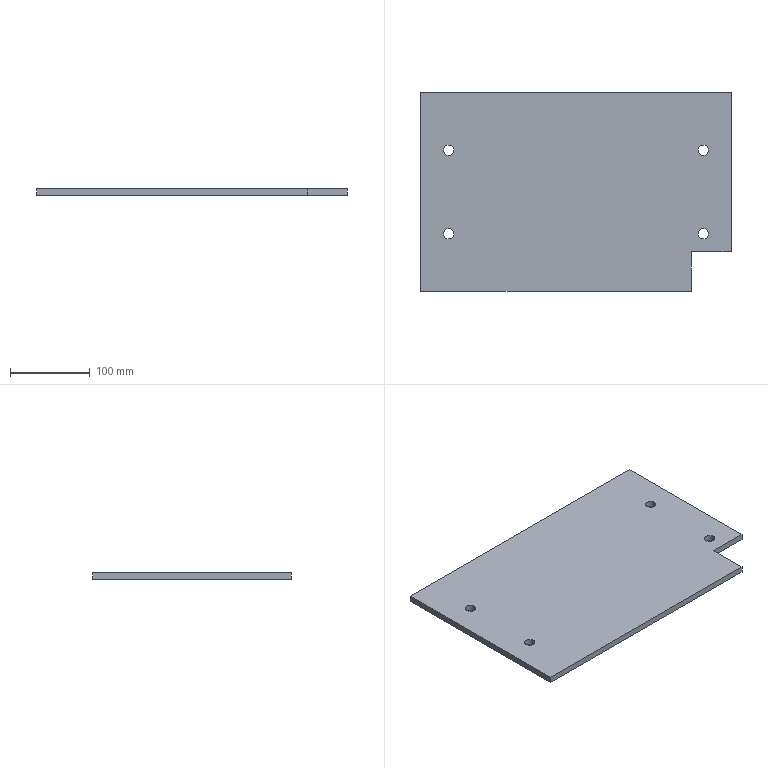Part | SolidWorks | features ICE 2, Extrusion 1 | 1 solid | 16 faces | box 390 x 250 x 8 mm | volume 755753 mm3 | cylinder 8 | plane 8 | commonest cylinder face diameters 13 x8
STEP:
#1=CARTESIAN_POINT('',(348.5,177.5,0.));
#2=VERTEX_POINT('',#1);
#3=CARTESIAN_POINT('',(361.5,177.5,0.));
#4=VERTEX_POINT('',#3);
#5=CARTESIAN_POINT('',(355.,177.5,0.));
#6=DIRECTION('',(0.,0.,1.));
#7=DIRECTION('',(1.,0.,0.));
#8=AXIS2_PLACEMENT_3D('',#5,#6,#7);
#9=CIRCLE('',#8,6.5);
#10=EDGE_CURVE('',#2,#4,#9,.T.);
#11=ORIENTED_EDGE('',*,*,#10,.F.);
#12=CARTESIAN_POINT('',(348.5,177.5,8.));
#13=VERTEX_POINT('',#12);
#14=CARTESIAN_POINT('',(348.5,177.5,0.));
#15=DIRECTION('',(0.,0.,1.));
#16=VECTOR('',#15,1000.);
#17=LINE('',#14,#16);
#18=EDGE_CURVE('',#2,#13,#17,.T.);
#19=ORIENTED_EDGE('',*,*,#18,.T.);
#20=CARTESIAN_POINT('',(361.5,177.5,8.));
#21=VERTEX_POINT('',#20);
#22=CARTESIAN_POINT('',(355.,177.5,8.));
#23=DIRECTION('',(0.,0.,1.));
#24=DIRECTION('',(1.,0.,0.));
#25=AXIS2_PLACEMENT_3D('',#22,#23,#24);
#26=CIRCLE('',#25,6.5);
#27=EDGE_CURVE('',#13,#21,#26,.T.);
#28=ORIENTED_EDGE('',*,*,#27,.T.);
#29=CARTESIAN_POINT('',(361.5,177.5,0.));
#30=DIRECTION('',(0.,0.,1.));
#31=VECTOR('',#30,1000.);
#32=LINE('',#29,#31);
#33=EDGE_CURVE('',#4,#21,#32,.T.);
#34=ORIENTED_EDGE('',*,*,#33,.F.);
#35=EDGE_LOOP('',(#11,#19,#28,#34));
#36=FACE_OUTER_BOUND('',#35,.T.);
#37=CARTESIAN_POINT('',(355.,177.5,0.));
#38=DIRECTION('',(0.,0.,1.));
#39=DIRECTION('',(1.,0.,0.));
#40=AXIS2_PLACEMENT_3D('',#37,#38,#39);
#41=CYLINDRICAL_SURFACE('',#40,6.5);
#42=ADVANCED_FACE('',(#36),#41,.F.);
#43=CARTESIAN_POINT('',(348.5,72.5,0.));
#44=VERTEX_POINT('',#43);
#45=CARTESIAN_POINT('',(361.5,72.5,0.));
#46=VERTEX_POINT('',#45);
#47=CARTESIAN_POINT('',(355.,72.5,0.));
#48=DIRECTION('',(0.,0.,1.));
#49=DIRECTION('',(1.,0.,0.));
#50=AXIS2_PLACEMENT_3D('',#47,#48,#49);
#51=CIRCLE('',#50,6.5);
#52=EDGE_CURVE('',#44,#46,#51,.T.);
#53=ORIENTED_EDGE('',*,*,#52,.F.);
#54=CARTESIAN_POINT('',(348.5,72.5,8.));
#55=VERTEX_POINT('',#54);
#56=CARTESIAN_POINT('',(348.5,72.5,0.));
#57=DIRECTION('',(0.,0.,1.));
#58=VECTOR('',#57,1000.);
#59=LINE('',#56,#58);
#60=EDGE_CURVE('',#44,#55,#59,.T.);
#61=ORIENTED_EDGE('',*,*,#60,.T.);
#62=CARTESIAN_POINT('',(361.5,72.5,8.));
#63=VERTEX_POINT('',#62);
#64=CARTESIAN_POINT('',(355.,72.5,8.));
#65=DIRECTION('',(0.,0.,1.));
#66=DIRECTION('',(1.,0.,0.));
#67=AXIS2_PLACEMENT_3D('',#64,#65,#66);
#68=CIRCLE('',#67,6.5);
#69=EDGE_CURVE('',#55,#63,#68,.T.);
#70=ORIENTED_EDGE('',*,*,#69,.T.);
#71=CARTESIAN_POINT('',(361.5,72.5,0.));
#72=DIRECTION('',(0.,0.,1.));
#73=VECTOR('',#72,1000.);
#74=LINE('',#71,#73);
#75=EDGE_CURVE('',#46,#63,#74,.T.);
#76=ORIENTED_EDGE('',*,*,#75,.F.);
#77=EDGE_LOOP('',(#53,#61,#70,#76));
#78=FACE_OUTER_BOUND('',#77,.T.);
#79=CARTESIAN_POINT('',(355.,72.5,0.));
#80=DIRECTION('',(0.,0.,1.));
#81=DIRECTION('',(1.,0.,0.));
#82=AXIS2_PLACEMENT_3D('',#79,#80,#81);
#83=CYLINDRICAL_SURFACE('',#82,6.5);
#84=ADVANCED_FACE('',(#78),#83,.F.);
#85=CARTESIAN_POINT('',(28.5,72.5,0.));
#86=VERTEX_POINT('',#85);
#87=CARTESIAN_POINT('',(41.5,72.5,0.));
#88=VERTEX_POINT('',#87);
#89=CARTESIAN_POINT('',(35.,72.5,0.));
#90=DIRECTION('',(0.,0.,1.));
#91=DIRECTION('',(1.,0.,0.));
#92=AXIS2_PLACEMENT_3D('',#89,#90,#91);
#93=CIRCLE('',#92,6.5);
#94=EDGE_CURVE('',#86,#88,#93,.T.);
#95=ORIENTED_EDGE('',*,*,#94,.F.);
#96=CARTESIAN_POINT('',(28.5,72.5,8.));
#97=VERTEX_POINT('',#96);
#98=CARTESIAN_POINT('',(28.5,72.5,0.));
#99=DIRECTION('',(0.,0.,1.));
#100=VECTOR('',#99,1000.);
#101=LINE('',#98,#100);
#102=EDGE_CURVE('',#86,#97,#101,.T.);
#103=ORIENTED_EDGE('',*,*,#102,.T.);
#104=CARTESIAN_POINT('',(41.5,72.5,8.));
#105=VERTEX_POINT('',#104);
#106=CARTESIAN_POINT('',(35.,72.5,8.));
#107=DIRECTION('',(0.,0.,1.));
#108=DIRECTION('',(1.,0.,0.));
#109=AXIS2_PLACEMENT_3D('',#106,#107,#108);
#110=CIRCLE('',#109,6.5);
#111=EDGE_CURVE('',#97,#105,#110,.T.);
#112=ORIENTED_EDGE('',*,*,#111,.T.);
#113=CARTESIAN_POINT('',(41.5,72.5,0.));
#114=DIRECTION('',(0.,0.,1.));
#115=VECTOR('',#114,1000.);
#116=LINE('',#113,#115);
#117=EDGE_CURVE('',#88,#105,#116,.T.);
#118=ORIENTED_EDGE('',*,*,#117,.F.);
#119=EDGE_LOOP('',(#95,#103,#112,#118));
#120=FACE_OUTER_BOUND('',#119,.T.);
#121=CARTESIAN_POINT('',(35.,72.5,0.));
#122=DIRECTION('',(0.,0.,1.));
#123=DIRECTION('',(1.,0.,0.));
#124=AXIS2_PLACEMENT_3D('',#121,#122,#123);
#125=CYLINDRICAL_SURFACE('',#124,6.5);
#126=ADVANCED_FACE('',(#120),#125,.F.);
#127=CARTESIAN_POINT('',(28.5,177.5,0.));
#128=VERTEX_POINT('',#127);
#129=CARTESIAN_POINT('',(41.5,177.5,0.));
#130=VERTEX_POINT('',#129);
#131=CARTESIAN_POINT('',(35.,177.5,0.));
#132=DIRECTION('',(0.,0.,1.));
#133=DIRECTION('',(1.,0.,0.));
#134=AXIS2_PLACEMENT_3D('',#131,#132,#133);
#135=CIRCLE('',#134,6.5);
#136=EDGE_CURVE('',#128,#130,#135,.T.);
#137=ORIENTED_EDGE('',*,*,#136,.F.);
#138=CARTESIAN_POINT('',(28.5,177.5,8.));
#139=VERTEX_POINT('',#138);
#140=CARTESIAN_POINT('',(28.5,177.5,0.));
#141=DIRECTION('',(0.,0.,1.));
#142=VECTOR('',#141,1000.);
#143=LINE('',#140,#142);
#144=EDGE_CURVE('',#128,#139,#143,.T.);
#145=ORIENTED_EDGE('',*,*,#144,.T.);
#146=CARTESIAN_POINT('',(41.5,177.5,8.));
#147=VERTEX_POINT('',#146);
#148=CARTESIAN_POINT('',(35.,177.5,8.));
#149=DIRECTION('',(0.,0.,1.));
#150=DIRECTION('',(1.,0.,0.));
#151=AXIS2_PLACEMENT_3D('',#148,#149,#150);
#152=CIRCLE('',#151,6.5);
#153=EDGE_CURVE('',#139,#147,#152,.T.);
#154=ORIENTED_EDGE('',*,*,#153,.T.);
#155=CARTESIAN_POINT('',(41.5,177.5,0.));
#156=DIRECTION('',(0.,0.,1.));
#157=VECTOR('',#156,1000.);
#158=LINE('',#155,#157);
#159=EDGE_CURVE('',#130,#147,#158,.T.);
#160=ORIENTED_EDGE('',*,*,#159,.F.);
#161=EDGE_LOOP('',(#137,#145,#154,#160));
#162=FACE_OUTER_BOUND('',#161,.T.);
#163=CARTESIAN_POINT('',(35.,177.5,0.));
#164=DIRECTION('',(0.,0.,1.));
#165=DIRECTION('',(1.,0.,0.));
#166=AXIS2_PLACEMENT_3D('',#163,#164,#165);
#167=CYLINDRICAL_SURFACE('',#166,6.5);
#168=ADVANCED_FACE('',(#162),#167,.F.);
#169=CARTESIAN_POINT('',(0.,0.,0.));
#170=VERTEX_POINT('',#169);
#171=CARTESIAN_POINT('',(340.,0.,0.));
#172=VERTEX_POINT('',#171);
#173=CARTESIAN_POINT('',(390.,0.,0.));
#174=DIRECTION('',(1.,0.,0.));
#175=VECTOR('',#174,1000.);
#176=LINE('',#173,#175);
#177=EDGE_CURVE('',#170,#172,#176,.T.);
#178=ORIENTED_EDGE('',*,*,#177,.T.);
#179=CARTESIAN_POINT('',(340.,0.,8.));
#180=VERTEX_POINT('',#179);
#181=CARTESIAN_POINT('',(340.,0.,-52.));
#182=DIRECTION('',(0.,0.,1.));
#183=VECTOR('',#182,1000.);
#184=LINE('',#181,#183);
#185=EDGE_CURVE('',#172,#180,#184,.T.);
#186=ORIENTED_EDGE('',*,*,#185,.T.);
#187=CARTESIAN_POINT('',(0.,0.,8.));
#188=VERTEX_POINT('',#187);
#189=CARTESIAN_POINT('',(390.,0.,8.));
#190=DIRECTION('',(1.,0.,0.));
#191=VECTOR('',#190,1000.);
#192=LINE('',#189,#191);
#193=EDGE_CURVE('',#188,#180,#192,.T.);
#194=ORIENTED_EDGE('',*,*,#193,.F.);
#195=CARTESIAN_POINT('',(0.,0.,8.));
#196=DIRECTION('',(0.,0.,-1.));
#197=VECTOR('',#196,1000.);
#198=LINE('',#195,#197);
#199=EDGE_CURVE('',#188,#170,#198,.T.);
#200=ORIENTED_EDGE('',*,*,#199,.T.);
#201=EDGE_LOOP('',(#178,#186,#194,#200));
#202=FACE_OUTER_BOUND('',#201,.T.);
#203=CARTESIAN_POINT('',(390.,0.,8.));
#204=DIRECTION('',(0.,1.,0.));
#205=DIRECTION('',(0.,0.,1.));
#206=AXIS2_PLACEMENT_3D('',#203,#204,#205);
#207=PLANE('',#206);
#208=ADVANCED_FACE('',(#202),#207,.F.);
#209=CARTESIAN_POINT('',(390.,50.,8.));
#210=VERTEX_POINT('',#209);
#211=CARTESIAN_POINT('',(390.,250.,8.));
#212=VERTEX_POINT('',#211);
#213=CARTESIAN_POINT('',(390.,250.,8.));
#214=DIRECTION('',(0.,1.,0.));
#215=VECTOR('',#214,1000.);
#216=LINE('',#213,#215);
#217=EDGE_CURVE('',#210,#212,#216,.T.);
#218=ORIENTED_EDGE('',*,*,#217,.F.);
#219=CARTESIAN_POINT('',(390.,50.,0.));
#220=VERTEX_POINT('',#219);
#221=CARTESIAN_POINT('',(390.,50.,-52.));
#222=DIRECTION('',(0.,0.,1.));
#223=VECTOR('',#222,1000.);
#224=LINE('',#221,#223);
#225=EDGE_CURVE('',#220,#210,#224,.T.);
#226=ORIENTED_EDGE('',*,*,#225,.F.);
#227=CARTESIAN_POINT('',(390.,250.,0.));
#228=VERTEX_POINT('',#227);
#229=CARTESIAN_POINT('',(390.,250.,0.));
#230=DIRECTION('',(0.,1.,0.));
#231=VECTOR('',#230,1000.);
#232=LINE('',#229,#231);
#233=EDGE_CURVE('',#220,#228,#232,.T.);
#234=ORIENTED_EDGE('',*,*,#233,.T.);
#235=CARTESIAN_POINT('',(390.,250.,8.));
#236=DIRECTION('',(0.,0.,-1.));
#237=VECTOR('',#236,1000.);
#238=LINE('',#235,#237);
#239=EDGE_CURVE('',#212,#228,#238,.T.);
#240=ORIENTED_EDGE('',*,*,#239,.F.);
#241=EDGE_LOOP('',(#218,#226,#234,#240));
#242=FACE_OUTER_BOUND('',#241,.T.);
#243=CARTESIAN_POINT('',(390.,250.,8.));
#244=DIRECTION('',(-1.,0.,0.));
#245=DIRECTION('',(0.,0.,1.));
#246=AXIS2_PLACEMENT_3D('',#243,#244,#245);
#247=PLANE('',#246);
#248=ADVANCED_FACE('',(#242),#247,.F.);
#249=CARTESIAN_POINT('',(0.,250.,0.));
#250=VERTEX_POINT('',#249);
#251=CARTESIAN_POINT('',(0.,250.,0.));
#252=DIRECTION('',(-1.,0.,0.));
#253=VECTOR('',#252,1000.);
#254=LINE('',#251,#253);
#255=EDGE_CURVE('',#228,#250,#254,.T.);
#256=ORIENTED_EDGE('',*,*,#255,.T.);
#257=CARTESIAN_POINT('',(0.,250.,8.));
#258=VERTEX_POINT('',#257);
#259=CARTESIAN_POINT('',(0.,250.,8.));
#260=DIRECTION('',(0.,0.,-1.));
#261=VECTOR('',#260,1000.);
#262=LINE('',#259,#261);
#263=EDGE_CURVE('',#258,#250,#262,.T.);
#264=ORIENTED_EDGE('',*,*,#263,.F.);
#265=CARTESIAN_POINT('',(0.,250.,8.));
#266=DIRECTION('',(-1.,0.,0.));
#267=VECTOR('',#266,1000.);
#268=LINE('',#265,#267);
#269=EDGE_CURVE('',#212,#258,#268,.T.);
#270=ORIENTED_EDGE('',*,*,#269,.F.);
#271=ORIENTED_EDGE('',*,*,#239,.T.);
#272=EDGE_LOOP('',(#256,#264,#270,#271));
#273=FACE_OUTER_BOUND('',#272,.T.);
#274=CARTESIAN_POINT('',(0.,250.,8.));
#275=DIRECTION('',(0.,-1.,0.));
#276=DIRECTION('',(0.,0.,-1.));
#277=AXIS2_PLACEMENT_3D('',#274,#275,#276);
#278=PLANE('',#277);
#279=ADVANCED_FACE('',(#273),#278,.F.);
#280=CARTESIAN_POINT('',(0.,0.,0.));
#281=DIRECTION('',(0.,-1.,0.));
#282=VECTOR('',#281,1000.);
#283=LINE('',#280,#282);
#284=EDGE_CURVE('',#250,#170,#283,.T.);
#285=ORIENTED_EDGE('',*,*,#284,.T.);
#286=ORIENTED_EDGE('',*,*,#199,.F.);
#287=CARTESIAN_POINT('',(0.,0.,8.));
#288=DIRECTION('',(0.,-1.,0.));
#289=VECTOR('',#288,1000.);
#290=LINE('',#287,#289);
#291=EDGE_CURVE('',#258,#188,#290,.T.);
#292=ORIENTED_EDGE('',*,*,#291,.F.);
#293=ORIENTED_EDGE('',*,*,#263,.T.);
#294=EDGE_LOOP('',(#285,#286,#292,#293));
#295=FACE_OUTER_BOUND('',#294,.T.);
#296=CARTESIAN_POINT('',(0.,0.,8.));
#297=DIRECTION('',(1.,0.,0.));
#298=DIRECTION('',(0.,0.,-1.));
#299=AXIS2_PLACEMENT_3D('',#296,#297,#298);
#300=PLANE('',#299);
#301=ADVANCED_FACE('',(#295),#300,.F.);
#302=CARTESIAN_POINT('',(355.,177.5,8.));
#303=DIRECTION('',(0.,0.,1.));
#304=DIRECTION('',(1.,0.,0.));
#305=AXIS2_PLACEMENT_3D('',#302,#303,#304);
#306=CIRCLE('',#305,6.5);
#307=EDGE_CURVE('',#21,#13,#306,.T.);
#308=ORIENTED_EDGE('',*,*,#307,.F.);
#309=ORIENTED_EDGE('',*,*,#27,.F.);
#310=EDGE_LOOP('',(#308,#309));
#311=FACE_BOUND('',#310,.T.);
#312=CARTESIAN_POINT('',(355.,72.5,8.));
#313=DIRECTION('',(0.,0.,1.));
#314=DIRECTION('',(1.,0.,0.));
#315=AXIS2_PLACEMENT_3D('',#312,#313,#314);
#316=CIRCLE('',#315,6.5);
#317=EDGE_CURVE('',#63,#55,#316,.T.);
#318=ORIENTED_EDGE('',*,*,#317,.F.);
#319=ORIENTED_EDGE('',*,*,#69,.F.);
#320=EDGE_LOOP('',(#318,#319));
#321=FACE_BOUND('',#320,.T.);
#322=CARTESIAN_POINT('',(35.,72.5,8.));
#323=DIRECTION('',(0.,0.,1.));
#324=DIRECTION('',(1.,0.,0.));
#325=AXIS2_PLACEMENT_3D('',#322,#323,#324);
#326=CIRCLE('',#325,6.5);
#327=EDGE_CURVE('',#105,#97,#326,.T.);
#328=ORIENTED_EDGE('',*,*,#327,.F.);
#329=ORIENTED_EDGE('',*,*,#111,.F.);
#330=EDGE_LOOP('',(#328,#329));
#331=FACE_BOUND('',#330,.T.);
#332=CARTESIAN_POINT('',(35.,177.5,8.));
#333=DIRECTION('',(0.,0.,1.));
#334=DIRECTION('',(1.,0.,0.));
#335=AXIS2_PLACEMENT_3D('',#332,#333,#334);
#336=CIRCLE('',#335,6.5);
#337=EDGE_CURVE('',#147,#139,#336,.T.);
#338=ORIENTED_EDGE('',*,*,#337,.F.);
#339=ORIENTED_EDGE('',*,*,#153,.F.);
#340=EDGE_LOOP('',(#338,#339));
#341=FACE_BOUND('',#340,.T.);
#342=ORIENTED_EDGE('',*,*,#193,.T.);
#343=CARTESIAN_POINT('',(340.,50.,8.));
#344=VERTEX_POINT('',#343);
#345=CARTESIAN_POINT('',(340.,0.,8.));
#346=DIRECTION('',(0.,-1.,0.));
#347=VECTOR('',#346,1000.);
#348=LINE('',#345,#347);
#349=EDGE_CURVE('',#344,#180,#348,.T.);
#350=ORIENTED_EDGE('',*,*,#349,.F.);
#351=CARTESIAN_POINT('',(340.,50.,8.));
#352=DIRECTION('',(-1.,0.,0.));
#353=VECTOR('',#352,1000.);
#354=LINE('',#351,#353);
#355=EDGE_CURVE('',#210,#344,#354,.T.);
#356=ORIENTED_EDGE('',*,*,#355,.F.);
#357=ORIENTED_EDGE('',*,*,#217,.T.);
#358=ORIENTED_EDGE('',*,*,#269,.T.);
#359=ORIENTED_EDGE('',*,*,#291,.T.);
#360=EDGE_LOOP('',(#342,#350,#356,#357,#358,#359));
#361=FACE_OUTER_BOUND('',#360,.T.);
#362=CARTESIAN_POINT('',(0.,0.,8.));
#363=DIRECTION('',(0.,0.,-1.));
#364=DIRECTION('',(-1.,0.,0.));
#365=AXIS2_PLACEMENT_3D('',#362,#363,#364);
#366=PLANE('',#365);
#367=ADVANCED_FACE('',(#311,#321,#331,#341,#361),#366,.F.);
#368=CARTESIAN_POINT('',(340.,50.,0.));
#369=VERTEX_POINT('',#368);
#370=CARTESIAN_POINT('',(340.,0.,0.));
#371=DIRECTION('',(0.,1.,0.));
#372=VECTOR('',#371,1000.);
#373=LINE('',#370,#372);
#374=EDGE_CURVE('',#172,#369,#373,.T.);
#375=ORIENTED_EDGE('',*,*,#374,.F.);
#376=ORIENTED_EDGE('',*,*,#177,.F.);
#377=ORIENTED_EDGE('',*,*,#284,.F.);
#378=ORIENTED_EDGE('',*,*,#255,.F.);
#379=ORIENTED_EDGE('',*,*,#233,.F.);
#380=CARTESIAN_POINT('',(0.,50.,0.));
#381=DIRECTION('',(1.,0.,0.));
#382=VECTOR('',#381,1000.);
#383=LINE('',#380,#382);
#384=EDGE_CURVE('',#369,#220,#383,.T.);
#385=ORIENTED_EDGE('',*,*,#384,.F.);
#386=EDGE_LOOP('',(#375,#376,#377,#378,#379,#385));
#387=FACE_OUTER_BOUND('',#386,.T.);
#388=CARTESIAN_POINT('',(355.,177.5,0.));
#389=DIRECTION('',(0.,0.,1.));
#390=DIRECTION('',(1.,0.,0.));
#391=AXIS2_PLACEMENT_3D('',#388,#389,#390);
#392=CIRCLE('',#391,6.5);
#393=EDGE_CURVE('',#4,#2,#392,.T.);
#394=ORIENTED_EDGE('',*,*,#393,.T.);
#395=ORIENTED_EDGE('',*,*,#10,.T.);
#396=EDGE_LOOP('',(#394,#395));
#397=FACE_BOUND('',#396,.T.);
#398=CARTESIAN_POINT('',(355.,72.5,0.));
#399=DIRECTION('',(0.,0.,1.));
#400=DIRECTION('',(1.,0.,0.));
#401=AXIS2_PLACEMENT_3D('',#398,#399,#400);
#402=CIRCLE('',#401,6.5);
#403=EDGE_CURVE('',#46,#44,#402,.T.);
#404=ORIENTED_EDGE('',*,*,#403,.T.);
#405=ORIENTED_EDGE('',*,*,#52,.T.);
#406=EDGE_LOOP('',(#404,#405));
#407=FACE_BOUND('',#406,.T.);
#408=CARTESIAN_POINT('',(35.,72.5,0.));
#409=DIRECTION('',(0.,0.,1.));
#410=DIRECTION('',(1.,0.,0.));
#411=AXIS2_PLACEMENT_3D('',#408,#409,#410);
#412=CIRCLE('',#411,6.5);
#413=EDGE_CURVE('',#88,#86,#412,.T.);
#414=ORIENTED_EDGE('',*,*,#413,.T.);
#415=ORIENTED_EDGE('',*,*,#94,.T.);
#416=EDGE_LOOP('',(#414,#415));
#417=FACE_BOUND('',#416,.T.);
#418=CARTESIAN_POINT('',(35.,177.5,0.));
#419=DIRECTION('',(0.,0.,1.));
#420=DIRECTION('',(1.,0.,0.));
#421=AXIS2_PLACEMENT_3D('',#418,#419,#420);
#422=CIRCLE('',#421,6.5);
#423=EDGE_CURVE('',#130,#128,#422,.T.);
#424=ORIENTED_EDGE('',*,*,#423,.T.);
#425=ORIENTED_EDGE('',*,*,#136,.T.);
#426=EDGE_LOOP('',(#424,#425));
#427=FACE_BOUND('',#426,.T.);
#428=CARTESIAN_POINT('',(0.,0.,0.));
#429=DIRECTION('',(0.,0.,-1.));
#430=DIRECTION('',(-1.,0.,0.));
#431=AXIS2_PLACEMENT_3D('',#428,#429,#430);
#432=PLANE('',#431);
#433=ADVANCED_FACE('',(#387,#397,#407,#417,#427),#432,.T.);
#434=ORIENTED_EDGE('',*,*,#144,.F.);
#435=ORIENTED_EDGE('',*,*,#423,.F.);
#436=ORIENTED_EDGE('',*,*,#159,.T.);
#437=ORIENTED_EDGE('',*,*,#337,.T.);
#438=EDGE_LOOP('',(#434,#435,#436,#437));
#439=FACE_OUTER_BOUND('',#438,.T.);
#440=CARTESIAN_POINT('',(35.,177.5,0.));
#441=DIRECTION('',(0.,0.,1.));
#442=DIRECTION('',(1.,0.,0.));
#443=AXIS2_PLACEMENT_3D('',#440,#441,#442);
#444=CYLINDRICAL_SURFACE('',#443,6.5);
#445=ADVANCED_FACE('',(#439),#444,.F.);
#446=ORIENTED_EDGE('',*,*,#102,.F.);
#447=ORIENTED_EDGE('',*,*,#413,.F.);
#448=ORIENTED_EDGE('',*,*,#117,.T.);
#449=ORIENTED_EDGE('',*,*,#327,.T.);
#450=EDGE_LOOP('',(#446,#447,#448,#449));
#451=FACE_OUTER_BOUND('',#450,.T.);
#452=CARTESIAN_POINT('',(35.,72.5,0.));
#453=DIRECTION('',(0.,0.,1.));
#454=DIRECTION('',(1.,0.,0.));
#455=AXIS2_PLACEMENT_3D('',#452,#453,#454);
#456=CYLINDRICAL_SURFACE('',#455,6.5);
#457=ADVANCED_FACE('',(#451),#456,.F.);
#458=ORIENTED_EDGE('',*,*,#60,.F.);
#459=ORIENTED_EDGE('',*,*,#403,.F.);
#460=ORIENTED_EDGE('',*,*,#75,.T.);
#461=ORIENTED_EDGE('',*,*,#317,.T.);
#462=EDGE_LOOP('',(#458,#459,#460,#461));
#463=FACE_OUTER_BOUND('',#462,.T.);
#464=CARTESIAN_POINT('',(355.,72.5,0.));
#465=DIRECTION('',(0.,0.,1.));
#466=DIRECTION('',(1.,0.,0.));
#467=AXIS2_PLACEMENT_3D('',#464,#465,#466);
#468=CYLINDRICAL_SURFACE('',#467,6.5);
#469=ADVANCED_FACE('',(#463),#468,.F.);
#470=ORIENTED_EDGE('',*,*,#18,.F.);
#471=ORIENTED_EDGE('',*,*,#393,.F.);
#472=ORIENTED_EDGE('',*,*,#33,.T.);
#473=ORIENTED_EDGE('',*,*,#307,.T.);
#474=EDGE_LOOP('',(#470,#471,#472,#473));
#475=FACE_OUTER_BOUND('',#474,.T.);
#476=CARTESIAN_POINT('',(355.,177.5,0.));
#477=DIRECTION('',(0.,0.,1.));
#478=DIRECTION('',(1.,0.,0.));
#479=AXIS2_PLACEMENT_3D('',#476,#477,#478);
#480=CYLINDRICAL_SURFACE('',#479,6.5);
#481=ADVANCED_FACE('',(#475),#480,.F.);
#482=ORIENTED_EDGE('',*,*,#374,.T.);
#483=CARTESIAN_POINT('',(340.,50.,-52.));
#484=DIRECTION('',(0.,0.,1.));
#485=VECTOR('',#484,1000.);
#486=LINE('',#483,#485);
#487=EDGE_CURVE('',#369,#344,#486,.T.);
#488=ORIENTED_EDGE('',*,*,#487,.T.);
#489=ORIENTED_EDGE('',*,*,#349,.T.);
#490=ORIENTED_EDGE('',*,*,#185,.F.);
#491=EDGE_LOOP('',(#482,#488,#489,#490));
#492=FACE_OUTER_BOUND('',#491,.T.);
#493=CARTESIAN_POINT('',(340.,0.,-52.));
#494=DIRECTION('',(-1.,0.,0.));
#495=DIRECTION('',(0.,0.,1.));
#496=AXIS2_PLACEMENT_3D('',#493,#494,#495);
#497=PLANE('',#496);
#498=ADVANCED_FACE('',(#492),#497,.F.);
#499=ORIENTED_EDGE('',*,*,#384,.T.);
#500=ORIENTED_EDGE('',*,*,#225,.T.);
#501=ORIENTED_EDGE('',*,*,#355,.T.);
#502=ORIENTED_EDGE('',*,*,#487,.F.);
#503=EDGE_LOOP('',(#499,#500,#501,#502));
#504=FACE_OUTER_BOUND('',#503,.T.);
#505=CARTESIAN_POINT('',(340.,50.,-52.));
#506=DIRECTION('',(0.,1.,0.));
#507=DIRECTION('',(0.,0.,1.));
#508=AXIS2_PLACEMENT_3D('',#505,#506,#507);
#509=PLANE('',#508);
#510=ADVANCED_FACE('',(#504),#509,.F.);
#511=CLOSED_SHELL('',(#42,#84,#126,#168,#208,#248,#279,#301,#367,#433,#445,#457,#469,#481,#498,#510));
#512=MANIFOLD_SOLID_BREP('',#511);
#513=CARTESIAN_POINT('',(0.,0.,0.));
#514=DIRECTION('',(0.,0.,1.));
#515=DIRECTION('',(1.,0.,0.));
#516=AXIS2_PLACEMENT_3D('',#513,#514,#515);
#517=(LENGTH_UNIT()NAMED_UNIT(*)SI_UNIT(.MILLI.,.METRE.));
#518=UNCERTAINTY_MEASURE_WITH_UNIT(LENGTH_MEASURE(0.00001),#517,'','');
#519=(NAMED_UNIT(*)PLANE_ANGLE_UNIT()SI_UNIT($,.RADIAN.));
#520=(NAMED_UNIT(*)SI_UNIT($,.STERADIAN.)SOLID_ANGLE_UNIT());
#521=(GEOMETRIC_REPRESENTATION_CONTEXT(3)GLOBAL_UNCERTAINTY_ASSIGNED_CONTEXT((#518))GLOBAL_UNIT_ASSIGNED_CONTEXT((#517,#519,#520))REPRESENTATION_CONTEXT('',''));
#522=ADVANCED_BREP_SHAPE_REPRESENTATION('',(#512,#516),#521);